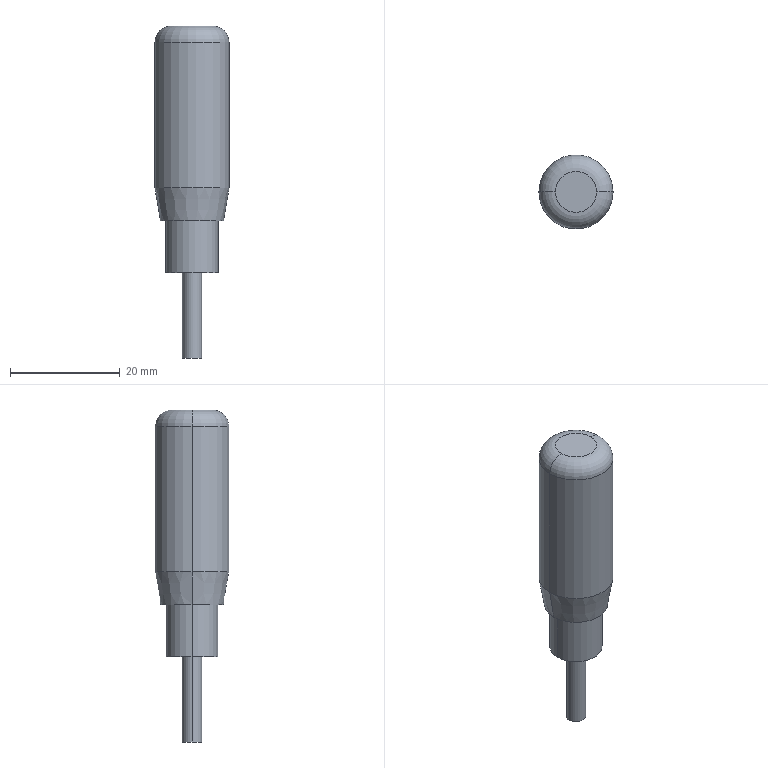Part | SolidWorks | features ICE 2, Chamfer 1, Extrusion 1, Fillet 1 | 1 solid | 14 faces | box 13.5 x 13.5 x 60.5 mm | volume 5709 mm3 | cylinder 6 | plane 4 | torus 2 | cone 2 | commonest cylinder face diameters 3.5 x2 9.5 x2 13.5 x2
STEP:
#1=CARTESIAN_POINT('',(-6.75,0.,57.5));
#2=VERTEX_POINT('',#1);
#3=CARTESIAN_POINT('',(6.75,0.,57.5));
#4=VERTEX_POINT('',#3);
#5=CARTESIAN_POINT('',(0.,0.,57.5));
#6=DIRECTION('',(0.,0.,-1.));
#7=DIRECTION('',(1.,0.,0.));
#8=AXIS2_PLACEMENT_3D('',#5,#6,#7);
#9=CIRCLE('',#8,6.75);
#10=EDGE_CURVE('',#2,#4,#9,.T.);
#11=ORIENTED_EDGE('',*,*,#10,.F.);
#12=CARTESIAN_POINT('',(-3.75,0.,60.5));
#13=VERTEX_POINT('',#12);
#14=CARTESIAN_POINT('',(-3.75,0.,57.5));
#15=DIRECTION('',(0.,1.,0.));
#16=DIRECTION('',(-1.,0.,0.));
#17=AXIS2_PLACEMENT_3D('',#14,#15,#16);
#18=CIRCLE('',#17,3.);
#19=EDGE_CURVE('',#2,#13,#18,.T.);
#20=ORIENTED_EDGE('',*,*,#19,.T.);
#21=CARTESIAN_POINT('',(3.75,0.,60.5));
#22=VERTEX_POINT('',#21);
#23=CARTESIAN_POINT('',(0.,0.,60.5));
#24=DIRECTION('',(0.,0.,1.));
#25=DIRECTION('',(1.,0.,0.));
#26=AXIS2_PLACEMENT_3D('',#23,#24,#25);
#27=CIRCLE('',#26,3.75);
#28=EDGE_CURVE('',#22,#13,#27,.T.);
#29=ORIENTED_EDGE('',*,*,#28,.F.);
#30=CARTESIAN_POINT('',(3.75,0.,57.5));
#31=DIRECTION('',(0.,-1.,0.));
#32=DIRECTION('',(0.,0.,-1.));
#33=AXIS2_PLACEMENT_3D('',#30,#31,#32);
#34=CIRCLE('',#33,3.);
#35=EDGE_CURVE('',#4,#22,#34,.T.);
#36=ORIENTED_EDGE('',*,*,#35,.F.);
#37=EDGE_LOOP('',(#11,#20,#29,#36));
#38=FACE_OUTER_BOUND('',#37,.T.);
#39=CARTESIAN_POINT('',(0.,0.,57.5));
#40=DIRECTION('',(0.,0.,1.));
#41=DIRECTION('',(1.,0.,0.));
#42=AXIS2_PLACEMENT_3D('',#39,#40,#41);
#43=TOROIDAL_SURFACE('',#42,3.75,3.);
#44=ADVANCED_FACE('',(#38),#43,.T.);
#45=CARTESIAN_POINT('',(-5.75,0.,25.));
#46=VERTEX_POINT('',#45);
#47=CARTESIAN_POINT('',(5.75,0.,25.));
#48=VERTEX_POINT('',#47);
#49=CARTESIAN_POINT('',(0.,0.,25.));
#50=DIRECTION('',(0.,0.,-1.));
#51=DIRECTION('',(1.,0.,0.));
#52=AXIS2_PLACEMENT_3D('',#49,#50,#51);
#53=CIRCLE('',#52,5.75);
#54=EDGE_CURVE('',#46,#48,#53,.T.);
#55=ORIENTED_EDGE('',*,*,#54,.F.);
#56=CARTESIAN_POINT('',(-6.75,0.,31.));
#57=VERTEX_POINT('',#56);
#58=CARTESIAN_POINT('',(-6.75,0.,31.));
#59=DIRECTION('',(-0.1644,0.,0.9864));
#60=VECTOR('',#59,1000.);
#61=LINE('',#58,#60);
#62=EDGE_CURVE('',#46,#57,#61,.T.);
#63=ORIENTED_EDGE('',*,*,#62,.T.);
#64=CARTESIAN_POINT('',(6.75,0.,31.));
#65=VERTEX_POINT('',#64);
#66=CARTESIAN_POINT('',(0.,0.,31.));
#67=DIRECTION('',(0.,0.,1.));
#68=DIRECTION('',(1.,0.,0.));
#69=AXIS2_PLACEMENT_3D('',#66,#67,#68);
#70=CIRCLE('',#69,6.75);
#71=EDGE_CURVE('',#65,#57,#70,.T.);
#72=ORIENTED_EDGE('',*,*,#71,.F.);
#73=CARTESIAN_POINT('',(6.75,0.,31.));
#74=DIRECTION('',(0.1644,0.,0.9864));
#75=VECTOR('',#74,1000.);
#76=LINE('',#73,#75);
#77=EDGE_CURVE('',#48,#65,#76,.T.);
#78=ORIENTED_EDGE('',*,*,#77,.F.);
#79=EDGE_LOOP('',(#55,#63,#72,#78));
#80=FACE_OUTER_BOUND('',#79,.T.);
#81=CARTESIAN_POINT('',(0.,0.,31.));
#82=DIRECTION('',(0.,0.,1.));
#83=DIRECTION('',(1.,0.,0.));
#84=AXIS2_PLACEMENT_3D('',#81,#82,#83);
#85=CONICAL_SURFACE('',#84,6.75,0.1651);
#86=ADVANCED_FACE('',(#80),#85,.T.);
#87=ORIENTED_EDGE('',*,*,#10,.T.);
#88=CARTESIAN_POINT('',(6.75,0.,60.5));
#89=DIRECTION('',(0.,0.,-1.));
#90=VECTOR('',#89,1000.);
#91=LINE('',#88,#90);
#92=EDGE_CURVE('',#4,#65,#91,.T.);
#93=ORIENTED_EDGE('',*,*,#92,.T.);
#94=ORIENTED_EDGE('',*,*,#71,.T.);
#95=CARTESIAN_POINT('',(-6.75,0.,60.5));
#96=DIRECTION('',(0.,0.,-1.));
#97=VECTOR('',#96,1000.);
#98=LINE('',#95,#97);
#99=EDGE_CURVE('',#2,#57,#98,.T.);
#100=ORIENTED_EDGE('',*,*,#99,.F.);
#101=EDGE_LOOP('',(#87,#93,#94,#100));
#102=FACE_OUTER_BOUND('',#101,.T.);
#103=CARTESIAN_POINT('',(0.,0.,60.5));
#104=DIRECTION('',(0.,0.,-1.));
#105=DIRECTION('',(-1.,0.,0.));
#106=AXIS2_PLACEMENT_3D('',#103,#104,#105);
#107=CYLINDRICAL_SURFACE('',#106,6.75);
#108=ADVANCED_FACE('',(#102),#107,.T.);
#109=CARTESIAN_POINT('',(4.75,0.,25.));
#110=VERTEX_POINT('',#109);
#111=CARTESIAN_POINT('',(-4.75,0.,25.));
#112=VERTEX_POINT('',#111);
#113=CARTESIAN_POINT('',(0.,0.,25.));
#114=DIRECTION('',(0.,0.,1.));
#115=DIRECTION('',(1.,0.,0.));
#116=AXIS2_PLACEMENT_3D('',#113,#114,#115);
#117=CIRCLE('',#116,4.75);
#118=EDGE_CURVE('',#110,#112,#117,.T.);
#119=ORIENTED_EDGE('',*,*,#118,.F.);
#120=CARTESIAN_POINT('',(4.75,0.,15.5));
#121=VERTEX_POINT('',#120);
#122=CARTESIAN_POINT('',(4.75,0.,25.));
#123=DIRECTION('',(0.,0.,-1.));
#124=VECTOR('',#123,1000.);
#125=LINE('',#122,#124);
#126=EDGE_CURVE('',#110,#121,#125,.T.);
#127=ORIENTED_EDGE('',*,*,#126,.T.);
#128=CARTESIAN_POINT('',(-4.75,0.,15.5));
#129=VERTEX_POINT('',#128);
#130=CARTESIAN_POINT('',(0.,0.,15.5));
#131=DIRECTION('',(0.,0.,1.));
#132=DIRECTION('',(1.,0.,0.));
#133=AXIS2_PLACEMENT_3D('',#130,#131,#132);
#134=CIRCLE('',#133,4.75);
#135=EDGE_CURVE('',#121,#129,#134,.T.);
#136=ORIENTED_EDGE('',*,*,#135,.T.);
#137=CARTESIAN_POINT('',(-4.75,0.,25.));
#138=DIRECTION('',(0.,0.,-1.));
#139=VECTOR('',#138,1000.);
#140=LINE('',#137,#139);
#141=EDGE_CURVE('',#112,#129,#140,.T.);
#142=ORIENTED_EDGE('',*,*,#141,.F.);
#143=EDGE_LOOP('',(#119,#127,#136,#142));
#144=FACE_OUTER_BOUND('',#143,.T.);
#145=CARTESIAN_POINT('',(0.,0.,25.));
#146=DIRECTION('',(0.,0.,-1.));
#147=DIRECTION('',(-1.,0.,0.));
#148=AXIS2_PLACEMENT_3D('',#145,#146,#147);
#149=CYLINDRICAL_SURFACE('',#148,4.75);
#150=ADVANCED_FACE('',(#144),#149,.T.);
#151=CARTESIAN_POINT('',(1.75,0.,15.5));
#152=VERTEX_POINT('',#151);
#153=CARTESIAN_POINT('',(-1.75,0.,15.5));
#154=VERTEX_POINT('',#153);
#155=CARTESIAN_POINT('',(0.,0.,15.5));
#156=DIRECTION('',(0.,0.,1.));
#157=DIRECTION('',(1.,0.,0.));
#158=AXIS2_PLACEMENT_3D('',#155,#156,#157);
#159=CIRCLE('',#158,1.75);
#160=EDGE_CURVE('',#152,#154,#159,.T.);
#161=ORIENTED_EDGE('',*,*,#160,.F.);
#162=CARTESIAN_POINT('',(1.75,0.,0.));
#163=VERTEX_POINT('',#162);
#164=CARTESIAN_POINT('',(1.75,0.,15.5));
#165=DIRECTION('',(0.,0.,-1.));
#166=VECTOR('',#165,1000.);
#167=LINE('',#164,#166);
#168=EDGE_CURVE('',#152,#163,#167,.T.);
#169=ORIENTED_EDGE('',*,*,#168,.T.);
#170=CARTESIAN_POINT('',(-1.75,0.,0.));
#171=VERTEX_POINT('',#170);
#172=CARTESIAN_POINT('',(0.,0.,0.));
#173=DIRECTION('',(0.,0.,1.));
#174=DIRECTION('',(1.,0.,0.));
#175=AXIS2_PLACEMENT_3D('',#172,#173,#174);
#176=CIRCLE('',#175,1.75);
#177=EDGE_CURVE('',#163,#171,#176,.T.);
#178=ORIENTED_EDGE('',*,*,#177,.T.);
#179=CARTESIAN_POINT('',(-1.75,0.,15.5));
#180=DIRECTION('',(0.,0.,-1.));
#181=VECTOR('',#180,1000.);
#182=LINE('',#179,#181);
#183=EDGE_CURVE('',#154,#171,#182,.T.);
#184=ORIENTED_EDGE('',*,*,#183,.F.);
#185=EDGE_LOOP('',(#161,#169,#178,#184));
#186=FACE_OUTER_BOUND('',#185,.T.);
#187=CARTESIAN_POINT('',(0.,0.,15.5));
#188=DIRECTION('',(0.,0.,-1.));
#189=DIRECTION('',(-1.,0.,0.));
#190=AXIS2_PLACEMENT_3D('',#187,#188,#189);
#191=CYLINDRICAL_SURFACE('',#190,1.75);
#192=ADVANCED_FACE('',(#186),#191,.T.);
#193=ORIENTED_EDGE('',*,*,#168,.F.);
#194=CARTESIAN_POINT('',(0.,0.,15.5));
#195=DIRECTION('',(0.,0.,1.));
#196=DIRECTION('',(1.,0.,0.));
#197=AXIS2_PLACEMENT_3D('',#194,#195,#196);
#198=CIRCLE('',#197,1.75);
#199=EDGE_CURVE('',#154,#152,#198,.T.);
#200=ORIENTED_EDGE('',*,*,#199,.F.);
#201=ORIENTED_EDGE('',*,*,#183,.T.);
#202=CARTESIAN_POINT('',(0.,0.,0.));
#203=DIRECTION('',(0.,0.,1.));
#204=DIRECTION('',(1.,0.,0.));
#205=AXIS2_PLACEMENT_3D('',#202,#203,#204);
#206=CIRCLE('',#205,1.75);
#207=EDGE_CURVE('',#171,#163,#206,.T.);
#208=ORIENTED_EDGE('',*,*,#207,.T.);
#209=EDGE_LOOP('',(#193,#200,#201,#208));
#210=FACE_OUTER_BOUND('',#209,.T.);
#211=CARTESIAN_POINT('',(0.,0.,15.5));
#212=DIRECTION('',(0.,0.,-1.));
#213=DIRECTION('',(-1.,0.,0.));
#214=AXIS2_PLACEMENT_3D('',#211,#212,#213);
#215=CYLINDRICAL_SURFACE('',#214,1.75);
#216=ADVANCED_FACE('',(#210),#215,.T.);
#217=ORIENTED_EDGE('',*,*,#207,.F.);
#218=ORIENTED_EDGE('',*,*,#177,.F.);
#219=EDGE_LOOP('',(#217,#218));
#220=FACE_OUTER_BOUND('',#219,.T.);
#221=CARTESIAN_POINT('',(0.,0.,0.));
#222=DIRECTION('',(0.,0.,1.));
#223=DIRECTION('',(1.,0.,0.));
#224=AXIS2_PLACEMENT_3D('',#221,#222,#223);
#225=PLANE('',#224);
#226=ADVANCED_FACE('',(#220),#225,.F.);
#227=CARTESIAN_POINT('',(0.,0.,15.5));
#228=DIRECTION('',(0.,0.,1.));
#229=DIRECTION('',(1.,0.,0.));
#230=AXIS2_PLACEMENT_3D('',#227,#228,#229);
#231=CIRCLE('',#230,4.75);
#232=EDGE_CURVE('',#129,#121,#231,.T.);
#233=ORIENTED_EDGE('',*,*,#232,.F.);
#234=ORIENTED_EDGE('',*,*,#135,.F.);
#235=EDGE_LOOP('',(#233,#234));
#236=FACE_OUTER_BOUND('',#235,.T.);
#237=ORIENTED_EDGE('',*,*,#199,.T.);
#238=ORIENTED_EDGE('',*,*,#160,.T.);
#239=EDGE_LOOP('',(#237,#238));
#240=FACE_BOUND('',#239,.T.);
#241=CARTESIAN_POINT('',(0.,0.,15.5));
#242=DIRECTION('',(0.,0.,1.));
#243=DIRECTION('',(1.,0.,0.));
#244=AXIS2_PLACEMENT_3D('',#241,#242,#243);
#245=PLANE('',#244);
#246=ADVANCED_FACE('',(#236,#240),#245,.F.);
#247=ORIENTED_EDGE('',*,*,#126,.F.);
#248=CARTESIAN_POINT('',(0.,0.,25.));
#249=DIRECTION('',(0.,0.,1.));
#250=DIRECTION('',(1.,0.,0.));
#251=AXIS2_PLACEMENT_3D('',#248,#249,#250);
#252=CIRCLE('',#251,4.75);
#253=EDGE_CURVE('',#112,#110,#252,.T.);
#254=ORIENTED_EDGE('',*,*,#253,.F.);
#255=ORIENTED_EDGE('',*,*,#141,.T.);
#256=ORIENTED_EDGE('',*,*,#232,.T.);
#257=EDGE_LOOP('',(#247,#254,#255,#256));
#258=FACE_OUTER_BOUND('',#257,.T.);
#259=CARTESIAN_POINT('',(0.,0.,25.));
#260=DIRECTION('',(0.,0.,-1.));
#261=DIRECTION('',(-1.,0.,0.));
#262=AXIS2_PLACEMENT_3D('',#259,#260,#261);
#263=CYLINDRICAL_SURFACE('',#262,4.75);
#264=ADVANCED_FACE('',(#258),#263,.T.);
#265=CARTESIAN_POINT('',(0.,0.,25.));
#266=DIRECTION('',(0.,0.,-1.));
#267=DIRECTION('',(1.,0.,0.));
#268=AXIS2_PLACEMENT_3D('',#265,#266,#267);
#269=CIRCLE('',#268,5.75);
#270=EDGE_CURVE('',#48,#46,#269,.T.);
#271=ORIENTED_EDGE('',*,*,#270,.T.);
#272=ORIENTED_EDGE('',*,*,#54,.T.);
#273=EDGE_LOOP('',(#271,#272));
#274=FACE_OUTER_BOUND('',#273,.T.);
#275=ORIENTED_EDGE('',*,*,#253,.T.);
#276=ORIENTED_EDGE('',*,*,#118,.T.);
#277=EDGE_LOOP('',(#275,#276));
#278=FACE_BOUND('',#277,.T.);
#279=CARTESIAN_POINT('',(0.,0.,25.));
#280=DIRECTION('',(0.,0.,1.));
#281=DIRECTION('',(1.,0.,0.));
#282=AXIS2_PLACEMENT_3D('',#279,#280,#281);
#283=PLANE('',#282);
#284=ADVANCED_FACE('',(#274,#278),#283,.F.);
#285=ORIENTED_EDGE('',*,*,#92,.F.);
#286=CARTESIAN_POINT('',(0.,0.,57.5));
#287=DIRECTION('',(0.,0.,-1.));
#288=DIRECTION('',(1.,0.,0.));
#289=AXIS2_PLACEMENT_3D('',#286,#287,#288);
#290=CIRCLE('',#289,6.75);
#291=EDGE_CURVE('',#4,#2,#290,.T.);
#292=ORIENTED_EDGE('',*,*,#291,.T.);
#293=ORIENTED_EDGE('',*,*,#99,.T.);
#294=CARTESIAN_POINT('',(0.,0.,31.));
#295=DIRECTION('',(0.,0.,1.));
#296=DIRECTION('',(1.,0.,0.));
#297=AXIS2_PLACEMENT_3D('',#294,#295,#296);
#298=CIRCLE('',#297,6.75);
#299=EDGE_CURVE('',#57,#65,#298,.T.);
#300=ORIENTED_EDGE('',*,*,#299,.T.);
#301=EDGE_LOOP('',(#285,#292,#293,#300));
#302=FACE_OUTER_BOUND('',#301,.T.);
#303=CARTESIAN_POINT('',(0.,0.,60.5));
#304=DIRECTION('',(0.,0.,-1.));
#305=DIRECTION('',(-1.,0.,0.));
#306=AXIS2_PLACEMENT_3D('',#303,#304,#305);
#307=CYLINDRICAL_SURFACE('',#306,6.75);
#308=ADVANCED_FACE('',(#302),#307,.T.);
#309=ORIENTED_EDGE('',*,*,#28,.T.);
#310=CARTESIAN_POINT('',(0.,0.,60.5));
#311=DIRECTION('',(0.,0.,1.));
#312=DIRECTION('',(1.,0.,0.));
#313=AXIS2_PLACEMENT_3D('',#310,#311,#312);
#314=CIRCLE('',#313,3.75);
#315=EDGE_CURVE('',#13,#22,#314,.T.);
#316=ORIENTED_EDGE('',*,*,#315,.T.);
#317=EDGE_LOOP('',(#309,#316));
#318=FACE_OUTER_BOUND('',#317,.T.);
#319=CARTESIAN_POINT('',(0.,0.,60.5));
#320=DIRECTION('',(0.,0.,1.));
#321=DIRECTION('',(1.,0.,0.));
#322=AXIS2_PLACEMENT_3D('',#319,#320,#321);
#323=PLANE('',#322);
#324=ADVANCED_FACE('',(#318),#323,.T.);
#325=ORIENTED_EDGE('',*,*,#62,.F.);
#326=ORIENTED_EDGE('',*,*,#270,.F.);
#327=ORIENTED_EDGE('',*,*,#77,.T.);
#328=ORIENTED_EDGE('',*,*,#299,.F.);
#329=EDGE_LOOP('',(#325,#326,#327,#328));
#330=FACE_OUTER_BOUND('',#329,.T.);
#331=CARTESIAN_POINT('',(0.,0.,31.));
#332=DIRECTION('',(0.,0.,1.));
#333=DIRECTION('',(1.,0.,0.));
#334=AXIS2_PLACEMENT_3D('',#331,#332,#333);
#335=CONICAL_SURFACE('',#334,6.75,0.1651);
#336=ADVANCED_FACE('',(#330),#335,.T.);
#337=ORIENTED_EDGE('',*,*,#19,.F.);
#338=ORIENTED_EDGE('',*,*,#291,.F.);
#339=ORIENTED_EDGE('',*,*,#35,.T.);
#340=ORIENTED_EDGE('',*,*,#315,.F.);
#341=EDGE_LOOP('',(#337,#338,#339,#340));
#342=FACE_OUTER_BOUND('',#341,.T.);
#343=CARTESIAN_POINT('',(0.,0.,57.5));
#344=DIRECTION('',(0.,0.,1.));
#345=DIRECTION('',(1.,0.,0.));
#346=AXIS2_PLACEMENT_3D('',#343,#344,#345);
#347=TOROIDAL_SURFACE('',#346,3.75,3.);
#348=ADVANCED_FACE('',(#342),#347,.T.);
#349=CLOSED_SHELL('',(#44,#86,#108,#150,#192,#216,#226,#246,#264,#284,#308,#324,#336,#348));
#350=MANIFOLD_SOLID_BREP('',#349);
#351=CARTESIAN_POINT('',(0.,0.,0.));
#352=DIRECTION('',(0.,0.,1.));
#353=DIRECTION('',(1.,0.,0.));
#354=AXIS2_PLACEMENT_3D('',#351,#352,#353);
#355=(LENGTH_UNIT()NAMED_UNIT(*)SI_UNIT(.MILLI.,.METRE.));
#356=UNCERTAINTY_MEASURE_WITH_UNIT(LENGTH_MEASURE(0.00001),#355,'','');
#357=(NAMED_UNIT(*)PLANE_ANGLE_UNIT()SI_UNIT($,.RADIAN.));
#358=(NAMED_UNIT(*)SI_UNIT($,.STERADIAN.)SOLID_ANGLE_UNIT());
#359=(GEOMETRIC_REPRESENTATION_CONTEXT(3)GLOBAL_UNCERTAINTY_ASSIGNED_CONTEXT((#356))GLOBAL_UNIT_ASSIGNED_CONTEXT((#355,#357,#358))REPRESENTATION_CONTEXT('',''));
#360=ADVANCED_BREP_SHAPE_REPRESENTATION('',(#350,#354),#359);